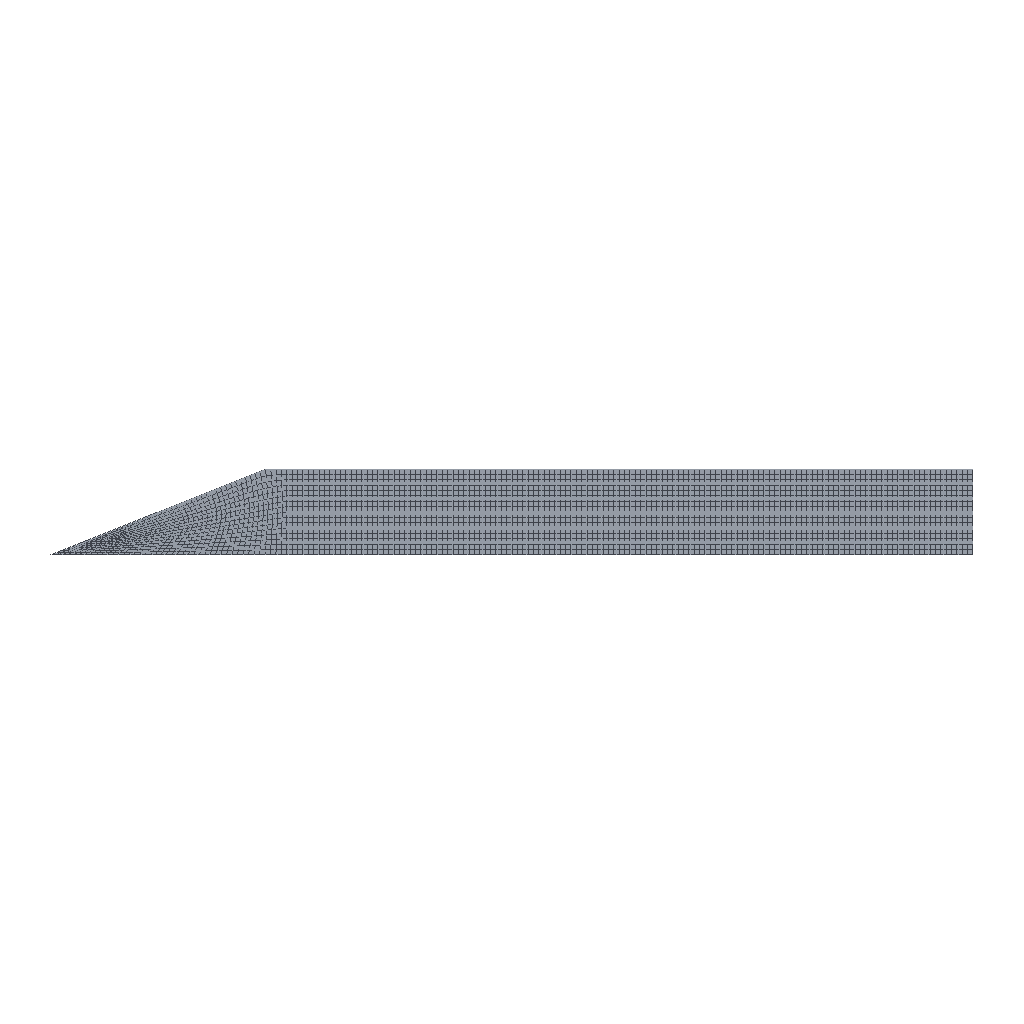Simulation study | abaqus
Set-up summary:
category,name,step,type,value,unit,region
solver,abaqus,,Abaqus/CAE 2024
units,mm-N-s-tonne (MPa),,inferred,E=20000 density=
analysis,gravity,,static,time_period=1
mesh,nodes,,,2882
mesh,elements,,,2700
element_type,CPE4,,,2700
material,concrete,,E,20000
material,concrete,,nu,0.3
material,soil,,E,20000
material,soil,,nu,0.3
section,concrete,,solid section,,,concrete
section,soil,,solid section,,,soil
load,Load-1,gravity,by,-20,,_PickedSet10
bc,BC-1,initial,fixed,"[dofs=x,y n=2]",,_PickedSet8
bc,BC-2,initial,fixed,[dofs=x],,_PickedSet9
Abaqus input file, long lists of numbers shortened:
*Heading
** Job name: deck Model name: Model-1
** Generated by: Abaqus/CAE 2024
*Preprint, echo=NO, model=NO, history=NO, contact=NO
**
** PARTS
**
*Part, name=Part-1
*Node
      1,          12.,           4.
      2,          12.,           3.
** (2880 more lines like these left out)
*Element, type=CPE4
 1,   1,  14, 414,  25
 2,  14,  15, 415, 414
** (2698 more lines like these left out)
*Nset, nset=concrete
    1,    2,    3,    4,    6,    8,   14,   15,   16,   17,   18,   19,   20,   21,   22,   23
   24,   25,  124,  125,  126,  402,  403,  404,  411,  412,  413,  414,  415,  416,  417,  418
** (1 more lines like these left out)
*Elset, elset=concrete
    1,    2,    3,    4,    5,    6,    7,    8,    9,   10,   11,   12,   13,   14,   15,   16
 2685, 2686, 2687, 2688, 2689, 2690, 2691, 2692, 2693, 2694, 2695, 2696, 2697, 2698, 2699, 2700
*Nset, nset=soil
    2,    3,    4,    5,    6,    7,    8,    9,   10,   11,   12,   13,   17,   18,   19,   20
   21,   22,   26,   27,   28,   29,   30,   31,   32,   33,   34,   35,   36,   37,   38,   39
** (177 more lines like these left out)
*Elset, elset=soil, generate
   17,  2684,     1
** Section: concrete
*Solid Section, elset=concrete, material=concrete
,
** Section: soil
*Solid Section, elset=soil, material=soil
,
*End Part
**
**
** ASSEMBLY
**
*Assembly, name=Assembly
**
*Instance, name=Part-1-1, part=Part-1
*End Instance
**
*Nset, nset=_PickedSet8, internal, instance=Part-1-1
   5,   9,  10,  11,  13,  26,  27,  28,  29,  30,  31,  32,  33,  34,  35,  36
  37,  38,  39,  40,  41,  42,  43,  44,  45,  46,  47,  48,  49,  50,  51,  52
** (9 more lines like these left out)
*Elset, elset=_PickedSet8, internal, instance=Part-1-1
   17,   18,   19,   20,   21,   22,   23,   24,   25,   26,   27,   28,   29,   30,   31,   32
   33,   34,   35,   36,   37,   38,   39,   40,   41,   42,   43,   44,   45,   46,   47,   48
** (9 more lines like these left out)
*Nset, nset=_PickedSet9, internal, instance=Part-1-1
  11,  12, 246, 247, 248, 249, 250, 251, 252, 253, 254, 255, 256, 257, 258, 259
 260,
*Elset, elset=_PickedSet9, internal, instance=Part-1-1, generate
  788,  2588,   120
*Nset, nset=_PickedSet10, internal, instance=Part-1-1, generate
    1,  2882,     1
*Elset, elset=_PickedSet10, internal, instance=Part-1-1, generate
    1,  2700,     1
*End Assembly
**
** MATERIALS
**
*Material, name=concrete
*Elastic
20000., 0.3
*Material, name=soil
*Elastic
20000., 0.3
**
** BOUNDARY CONDITIONS
**
** Name: BC-1 Type: Displacement/Rotation
*Boundary
_PickedSet8, 1, 1
_PickedSet8, 2, 2
** Name: BC-2 Type: Displacement/Rotation
*Boundary
_PickedSet9, 1, 1
** ----------------------------------------------------------------
**
** STEP: gravity
**
*Step, name=gravity, nlgeom=NO
*Static
1., 1., 1e-05, 1.
**
** LOADS
**
** Name: Load-1   Type: Body force
*Dload
_PickedSet10, BY, -20.
**
** OUTPUT REQUESTS
**
*Restart, write, frequency=0
**
** FIELD OUTPUT: F-Output-1
**
*Output, field, variable=PRESELECT
**
** HISTORY OUTPUT: H-Output-1
**
*Output, history, variable=PRESELECT
*End Step
Results summary:
result,odb.job_status,,,JOB_STATUS_COMPLETED_SUCCESSFULLY,"consistent, unstated (Abaqus has no unit system)"
result,steps[0].procedure,gravity,,*STATIC,"consistent, unstated (Abaqus has no unit system)"
result,steps[0].time_period,gravity,,1,"consistent, unstated (Abaqus has no unit system)"
result,steps[0].n_frames,gravity,,2,"consistent, unstated (Abaqus has no unit system)"
result,steps[0].last_frame.id,gravity,,1,"consistent, unstated (Abaqus has no unit system)"
result,steps[0].last_frame.value,gravity,,1,"consistent, unstated (Abaqus has no unit system)"
result,steps[0].last_frame.description,gravity,,Increment      1: Step Time =    1.000,"consistent, unstated (Abaqus has no unit system)"
result,steps[0].completed,gravity,,True,"consistent, unstated (Abaqus has no unit system)"
result,steps[0].max_U_magnitude,gravity,,0.006028,"consistent, unstated (Abaqus has no unit system)"
result,steps[0].max_S_mises,gravity,,44.327,"consistent, unstated (Abaqus has no unit system)"
result,steps[0].RF_sum[1],gravity,,-5.06639e-06,"consistent, unstated (Abaqus has no unit system)"
result,steps[0].RF_sum[2],gravity,,3040,"consistent, unstated (Abaqus has no unit system)"